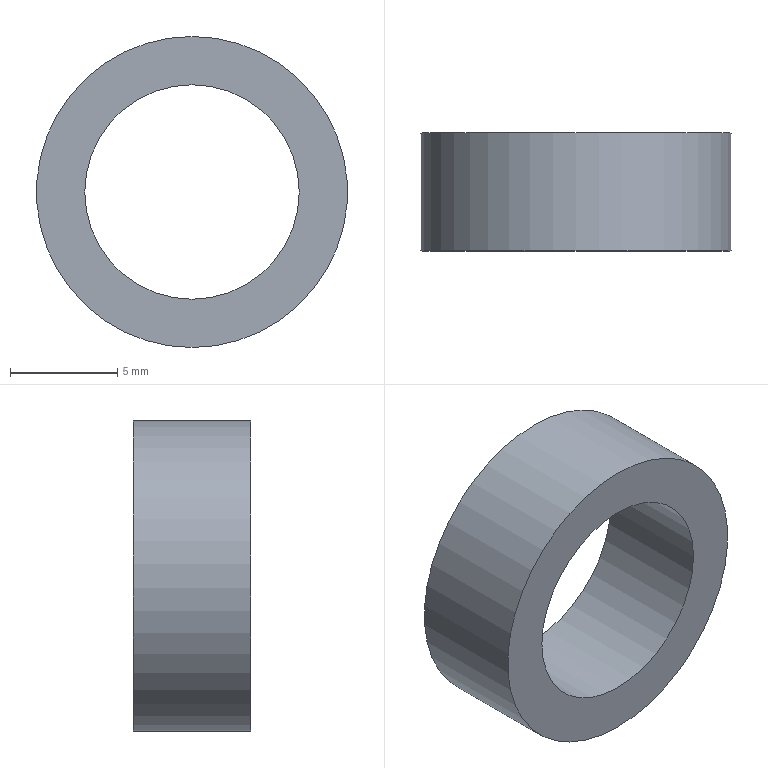Part | STEP file | ROTATION MC_NEW VER-0610_486 | 1 solid | 4 faces | box 14.5 x 5.5 x 14.5 mm | volume 476.246 mm3 | plane 2 | cylinder 2 | commonest cylinder face diameters 10 x1 14.5 x1
STEP:
#1=CARTESIAN_POINT('',(-232.469,678.468,-93.341));
#2=VERTEX_POINT('',#1);
#3=CARTESIAN_POINT('',(-232.469,678.468,-78.841));
#4=VERTEX_POINT('',#3);
#5=CARTESIAN_POINT('',(-232.469,678.468,-86.091));
#6=DIRECTION('',(0.,1.,0.));
#7=DIRECTION('',(0.,0.,-1.));
#8=AXIS2_PLACEMENT_3D('',#5,#6,#7);
#9=CIRCLE('',#8,7.25);
#10=EDGE_CURVE('',#2,#4,#9,.T.);
#11=ORIENTED_EDGE('',*,*,#10,.F.);
#12=CARTESIAN_POINT('',(-232.469,678.468,-86.091));
#13=DIRECTION('',(0.,1.,0.));
#14=DIRECTION('',(0.,0.,-1.));
#15=AXIS2_PLACEMENT_3D('',#12,#13,#14);
#16=CIRCLE('',#15,7.25);
#17=EDGE_CURVE('',#4,#2,#16,.T.);
#18=ORIENTED_EDGE('',*,*,#17,.F.);
#19=EDGE_LOOP('',(#11,#18));
#20=FACE_OUTER_BOUND('',#19,.T.);
#21=CARTESIAN_POINT('',(-232.469,678.468,-91.091));
#22=VERTEX_POINT('',#21);
#23=CARTESIAN_POINT('',(-232.469,678.468,-81.091));
#24=VERTEX_POINT('',#23);
#25=CARTESIAN_POINT('',(-232.469,678.468,-86.091));
#26=DIRECTION('',(0.,1.,0.));
#27=DIRECTION('',(0.,0.,-1.));
#28=AXIS2_PLACEMENT_3D('',#25,#26,#27);
#29=CIRCLE('',#28,5.);
#30=EDGE_CURVE('',#22,#24,#29,.T.);
#31=ORIENTED_EDGE('',*,*,#30,.T.);
#32=CARTESIAN_POINT('',(-232.469,678.468,-86.091));
#33=DIRECTION('',(0.,1.,0.));
#34=DIRECTION('',(0.,0.,-1.));
#35=AXIS2_PLACEMENT_3D('',#32,#33,#34);
#36=CIRCLE('',#35,5.);
#37=EDGE_CURVE('',#24,#22,#36,.T.);
#38=ORIENTED_EDGE('',*,*,#37,.T.);
#39=EDGE_LOOP('',(#31,#38));
#40=FACE_BOUND('',#39,.T.);
#41=CARTESIAN_POINT('',(-232.469,678.468,-86.091));
#42=DIRECTION('',(0.,1.,0.));
#43=DIRECTION('',(0.,0.,1.));
#44=AXIS2_PLACEMENT_3D('',#41,#42,#43);
#45=PLANE('',#44);
#46=ADVANCED_FACE('',(#20,#40),#45,.F.);
#47=CARTESIAN_POINT('',(-232.469,683.968,-93.341));
#48=VERTEX_POINT('',#47);
#49=CARTESIAN_POINT('',(-232.469,683.968,-78.841));
#50=VERTEX_POINT('',#49);
#51=CARTESIAN_POINT('',(-232.469,683.968,-86.091));
#52=DIRECTION('',(0.,1.,0.));
#53=DIRECTION('',(0.,0.,-1.));
#54=AXIS2_PLACEMENT_3D('',#51,#52,#53);
#55=CIRCLE('',#54,7.25);
#56=EDGE_CURVE('',#48,#50,#55,.T.);
#57=ORIENTED_EDGE('',*,*,#56,.T.);
#58=CARTESIAN_POINT('',(-232.469,683.968,-86.091));
#59=DIRECTION('',(0.,1.,0.));
#60=DIRECTION('',(0.,0.,-1.));
#61=AXIS2_PLACEMENT_3D('',#58,#59,#60);
#62=CIRCLE('',#61,7.25);
#63=EDGE_CURVE('',#50,#48,#62,.T.);
#64=ORIENTED_EDGE('',*,*,#63,.T.);
#65=EDGE_LOOP('',(#57,#64));
#66=FACE_OUTER_BOUND('',#65,.T.);
#67=CARTESIAN_POINT('',(-232.469,683.968,-91.091));
#68=VERTEX_POINT('',#67);
#69=CARTESIAN_POINT('',(-232.469,683.968,-81.091));
#70=VERTEX_POINT('',#69);
#71=CARTESIAN_POINT('',(-232.469,683.968,-86.091));
#72=DIRECTION('',(0.,1.,0.));
#73=DIRECTION('',(0.,0.,-1.));
#74=AXIS2_PLACEMENT_3D('',#71,#72,#73);
#75=CIRCLE('',#74,5.);
#76=EDGE_CURVE('',#68,#70,#75,.T.);
#77=ORIENTED_EDGE('',*,*,#76,.F.);
#78=CARTESIAN_POINT('',(-232.469,683.968,-86.091));
#79=DIRECTION('',(0.,1.,0.));
#80=DIRECTION('',(0.,0.,-1.));
#81=AXIS2_PLACEMENT_3D('',#78,#79,#80);
#82=CIRCLE('',#81,5.);
#83=EDGE_CURVE('',#70,#68,#82,.T.);
#84=ORIENTED_EDGE('',*,*,#83,.F.);
#85=EDGE_LOOP('',(#77,#84));
#86=FACE_BOUND('',#85,.T.);
#87=CARTESIAN_POINT('',(-232.469,683.968,-86.091));
#88=DIRECTION('',(0.,1.,0.));
#89=DIRECTION('',(0.,0.,1.));
#90=AXIS2_PLACEMENT_3D('',#87,#88,#89);
#91=PLANE('',#90);
#92=ADVANCED_FACE('',(#66,#86),#91,.T.);
#93=ORIENTED_EDGE('',*,*,#10,.T.);
#94=CARTESIAN_POINT('',(-232.469,683.968,-78.841));
#95=DIRECTION('',(0.,1.,0.));
#96=VECTOR('',#95,7.25);
#97=LINE('',#94,#96);
#98=EDGE_CURVE('',#4,#50,#97,.T.);
#99=ORIENTED_EDGE('',*,*,#98,.T.);
#100=ORIENTED_EDGE('',*,*,#56,.F.);
#101=ORIENTED_EDGE('',*,*,#63,.F.);
#102=ORIENTED_EDGE('',*,*,#98,.F.);
#103=ORIENTED_EDGE('',*,*,#17,.T.);
#104=EDGE_LOOP('',(#93,#99,#100,#101,#102,#103));
#105=FACE_OUTER_BOUND('',#104,.T.);
#106=CARTESIAN_POINT('',(-232.469,683.968,-86.091));
#107=DIRECTION('',(0.,-1.,0.));
#108=DIRECTION('',(0.,0.,-1.));
#109=AXIS2_PLACEMENT_3D('',#106,#107,#108);
#110=CYLINDRICAL_SURFACE('',#109,7.25);
#111=ADVANCED_FACE('',(#105),#110,.T.);
#112=ORIENTED_EDGE('',*,*,#76,.T.);
#113=CARTESIAN_POINT('',(-232.469,683.968,-81.091));
#114=DIRECTION('',(0.,-1.,0.));
#115=VECTOR('',#114,5.);
#116=LINE('',#113,#115);
#117=EDGE_CURVE('',#70,#24,#116,.T.);
#118=ORIENTED_EDGE('',*,*,#117,.T.);
#119=ORIENTED_EDGE('',*,*,#30,.F.);
#120=ORIENTED_EDGE('',*,*,#37,.F.);
#121=ORIENTED_EDGE('',*,*,#117,.F.);
#122=ORIENTED_EDGE('',*,*,#83,.T.);
#123=EDGE_LOOP('',(#112,#118,#119,#120,#121,#122));
#124=FACE_OUTER_BOUND('',#123,.T.);
#125=CARTESIAN_POINT('',(-232.469,683.968,-86.091));
#126=DIRECTION('',(0.,-1.,0.));
#127=DIRECTION('',(0.,0.,-1.));
#128=AXIS2_PLACEMENT_3D('',#125,#126,#127);
#129=CYLINDRICAL_SURFACE('',#128,5.);
#130=ADVANCED_FACE('',(#124),#129,.F.);
#131=CLOSED_SHELL('',(#46,#92,#111,#130));
#132=MANIFOLD_SOLID_BREP('',#131);
#133=(LENGTH_UNIT()NAMED_UNIT(*)SI_UNIT(.MILLI.,.METRE.));
#134=UNCERTAINTY_MEASURE_WITH_UNIT(LENGTH_MEASURE(0.01),#133,'','');
#135=(NAMED_UNIT(*)PLANE_ANGLE_UNIT()SI_UNIT($,.RADIAN.));
#136=(NAMED_UNIT(*)SI_UNIT($,.STERADIAN.)SOLID_ANGLE_UNIT());
#137=(GEOMETRIC_REPRESENTATION_CONTEXT(3)GLOBAL_UNCERTAINTY_ASSIGNED_CONTEXT((#134))GLOBAL_UNIT_ASSIGNED_CONTEXT((#133,#135,#136))REPRESENTATION_CONTEXT('',''));
#138=ADVANCED_BREP_SHAPE_REPRESENTATION('',(#132),#137);